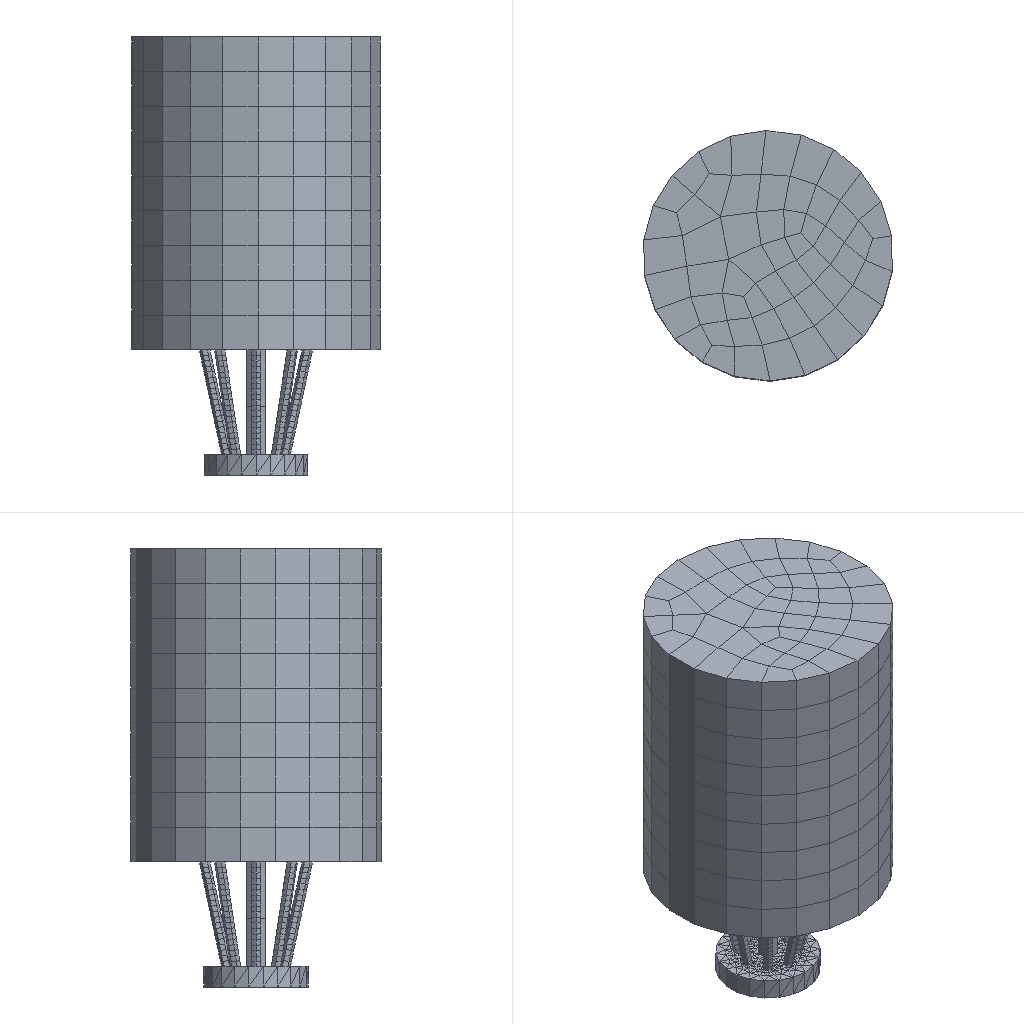Simulation study | abaqus
Set-up summary:
category,name,step,type,value,unit,region
solver,abaqus
solver,version,,,Abaqus/Standard 2020
units,not stated in the deck,,not stated
analysis,deck,,modal,modal
load_step,Step-1,Step-1,modal
load_step,requested,,,1
mesh,nodes,,,8569
mesh,elements,,,4242
element_type,C3D8,,solid,1718
element_type,C3D10,,solid,2524
load,load commands in deck,,count,0
bc,support commands in deck,,count,3
material,CON,,in results
material,SOIL,,in results
check,setup vs results,,match,"per instance, exact: element labels, types and connectivity; labels of the nodes the elements use; coordinates of those nodes at SINGLE_PRECISION in 2 of 3 instance(s)"
Abaqus input file, long lists of numbers shortened:
*Heading
** Job name: Job-1 Model name: Model-1
** Generated by: Abaqus/CAE 2020
*Preprint, echo=NO, model=NO, history=NO, contact=NO
**
** PARTS
**
*Part, name=Part-3
*Node
      1,   3.383,  -3.971,          12.
      2,   1.788,  -2.376,   1.388
** (3727 more lines like these left out)
*Element, type=C3D8
 1, 174, 173, 172, 169,   1,  36,  35,  32
 2, 172, 171, 170, 169,  35,  34,  33,  32
** (1230 more lines like these left out)
*Nset, nset=Set-2, generate
    1,  3729,     1
*Elset, elset=Set-2, generate
    1,  1232,     1
** Section: con
*Solid Section, elset=Set-2, material=con
,
*End Part
**
*Part, name=cut-chengtai
*Node
      1,   1.788,  -2.376,   1.388
      2,  -2.376,  -1.788,   1.388
** (4178 more lines like these left out)
*Element, type=C3D10
   1,  398,  158,  399,  400,  634,  633,  632,  636,  635,  637
   2,  401,  402,  302,  403,  640,  639,  638,  642,  641,  643
** (2522 more lines like these left out)
*Nset, nset=Set-4, generate
    1,  4180,     1
*Elset, elset=Set-4, generate
    1,  2524,     1
** Section: con
*Solid Section, elset=Set-4, material=con
,
*End Part
**
*Part, name=soil
*Node
      1,   9.2,   -7.705,           0.
      2,   10.998,   -4.801,           0.
** (658 more lines like these left out)
*Element, type=C3D8
  1,  89,  86,  85,  90,  23,  20,  19,  24
  2,  90,  85,  84,  91,  24,  19,  18,  25
** (484 more lines like these left out)
*Nset, nset=Set-2, generate
   1,  660,    1
*Elset, elset=Set-2, generate
   1,  486,    1
** Section: soil
*Solid Section, elset=Set-2, material=soil
,
*End Part
**
**
** ASSEMBLY
**
*Assembly, name=Assembly
**
*Instance, name=soil-1, part=soil
          0.,           0.,          12.
*End Instance
**
*Instance, name=cut-chengtai-1, part=cut-chengtai
*End Instance
**
*Instance, name=Part-3-1, part=Part-3
*End Instance
**
*Nset, nset=Set-3, instance=soil-1, generate
 595,  660,    1
*Elset, elset=Set-3, instance=soil-1, generate
 433,  486,    1
*Nset, nset=Set-4, instance=soil-1
   1,   2,   3,   4,   5,   6,   7,   8,   9,  10,  11,  12,  13,  14,  15,  16
  17,  18,  19,  20,  21,  22,  67,  68,  69,  70,  71,  72,  73,  74,  75,  76
** (12 more lines like these left out)
*Elset, elset=Set-4, instance=soil-1
   1,   2,   3,   4,  13,  14,  15,  16,  17,  18,  19,  20,  22,  23,  24,  25
  26,  27,  28,  29,  48,  49,  55,  56,  57,  58,  67,  68,  69,  70,  71,  72
** (11 more lines like these left out)
*Nset, nset=Set-5, instance=soil-1, generate
 595,  660,    1
*Elset, elset=Set-5, instance=soil-1, generate
 433,  486,    1
*Nset, nset=m_Set-1, instance=Part-3-1
    1,    3,    4,    6,    7,   10,   11,   13,   14,   17,   18,   20,   21,   24,   25,   27
   28,   31,   32,   33,   34,   35,   36,   42,   43,   44,   45,   46,   47,   48,   49,   50
** (170 more lines like these left out)
*Elset, elset=m_Set-1, instance=Part-3-1
   41,   42,   43,   44,   45,   46,   47,   48,   49,   50,   51,   52,   53,   54,   55,   56
   57,   58,   59,   60,   61,   62,   63,   64,   65,   66,   67,   68,   69,   70,   71,   72
** (55 more lines like these left out)
*Nset, nset=s_Set-1, instance=soil-1, generate
   1,  660,    1
*Elset, elset=s_Set-1, instance=soil-1, generate
   1,  486,    1
*Elset, elset=_m_Surf-1_S3, internal, instance=Part-3-1
    1,    2,    3,    4,    5,    6,    7,    8,    9,   10,   11,   12,   13,   14,   15,   16
   17,   18,   19,   20,   21,   22,   23,   24,   25,   26,   27,   28,   29,   30,   31,   32
** (19 more lines like these left out)
*Elset, elset=_m_Surf-1_S4, internal, instance=Part-3-1
    1,    2,    3,    4,    5,    6,    7,    8,    9,   10,   11,   12,   13,   14,   15,   16
   17,   18,   19,   20,   21,   22,   23,   24,   25,   26,   27,   28,   29,   30,   31,   32
** (14 more lines like these left out)
*Elset, elset=_m_Surf-1_S6, internal, instance=Part-3-1
    1,    3,    5,    7,    9,   11,   13,   15,   17,   19,   21,   23,   25,   27,   29,   31
   33,   35,   37,   39,  151,  153,  155,  157,  183,  184,  185,  186,  187,  188,  189,  190
** (14 more lines like these left out)
*Elset, elset=_m_Surf-1_S5, internal, instance=Part-3-1
    2,    4,    6,    8,   10,   12,   14,   16,   18,   20,   22,   24,   26,   28,   30,   32
   34,   36,   38,   40,  152,  154,  156,  158,  183,  185,  187,  189,  191,  193,  195,  197
** (9 more lines like these left out)
*Elset, elset=_m_Surf-1_S1, internal, instance=Part-3-1
   39,   40,  155,  156,  157,  158,  221,  222,  371,  372,  521,  522,  671,  672,  821,  822
  971,  972, 1121, 1122
*Surface, type=ELEMENT, name=m_Surf-1
_m_Surf-1_S3, S3
_m_Surf-1_S4, S4
_m_Surf-1_S6, S6
_m_Surf-1_S5, S5
_m_Surf-1_S1, S1
*Elset, elset=_s_Surf-1_S3, internal, instance=cut-chengtai-1
  128,  163,  233,  237,  241,  248,  251,  261,  271,  281,  288,  313,  343,  377,  389,  427
  490,  532,  544,  569,  604,  617,  851,  853,  985, 1075, 1179, 1253, 1306, 1386, 1518, 1538
** (12 more lines like these left out)
*Elset, elset=_s_Surf-1_S2, internal, instance=cut-chengtai-1
  229,  744,  778, 1056, 1759, 1942, 2086, 2088, 2103, 2184, 2234, 2262, 2288, 2326
*Elset, elset=_s_Surf-1_S4, internal, instance=cut-chengtai-1
  162,  280,  398, 1719, 1825, 1865, 1873, 2032, 2194
*Elset, elset=_s_Surf-1_S1, internal, instance=cut-chengtai-1
  884, 1120, 1401, 1981, 2136
*Surface, type=ELEMENT, name=s_Surf-1
_s_Surf-1_S3, S3
_s_Surf-1_S2, S2
_s_Surf-1_S4, S4
_s_Surf-1_S1, S1
** Constraint: Constraint-1
*Embedded Element, host elset=s_Set-1
m_Set-1
** Constraint: Constraint-2
*Tie, name=Constraint-2, adjust=yes
s_Surf-1, m_Surf-1
*End Assembly
**
** MATERIALS
**
*Material, name=con
*Density
2770.,
*Elastic
27450., 0.2
*Material, name=soil
*Density
2500.,
*Elastic
 1.3e+10, 0.35
**
** BOUNDARY CONDITIONS
**
** Name: BC-2 Type: 位移/转角
*Boundary
Set-4, 1, 1
Set-4, 2, 2
** Name: BC-3 Type: 位移/转角
*Boundary
Set-5, 3, 3
** ----------------------------------------------------------------
**
** STEP: Step-1
**
*Step, name=Step-1, nlgeom=NO, perturbation
*Frequency, eigensolver=Lanczos, sim, acoustic coupling=on, normalization=mass
8, , , , ,
**
** OUTPUT REQUESTS
**
*Restart, write, frequency=0
**
** FIELD OUTPUT: F-Output-1
**
*Output, field, variable=PRESELECT
*End Step
Results summary:
result,step,,partial,increments=0 time=0.0/1e-36
result,analysis,,,modal
result,last_loadstep,,,1
result,primary field,,,U